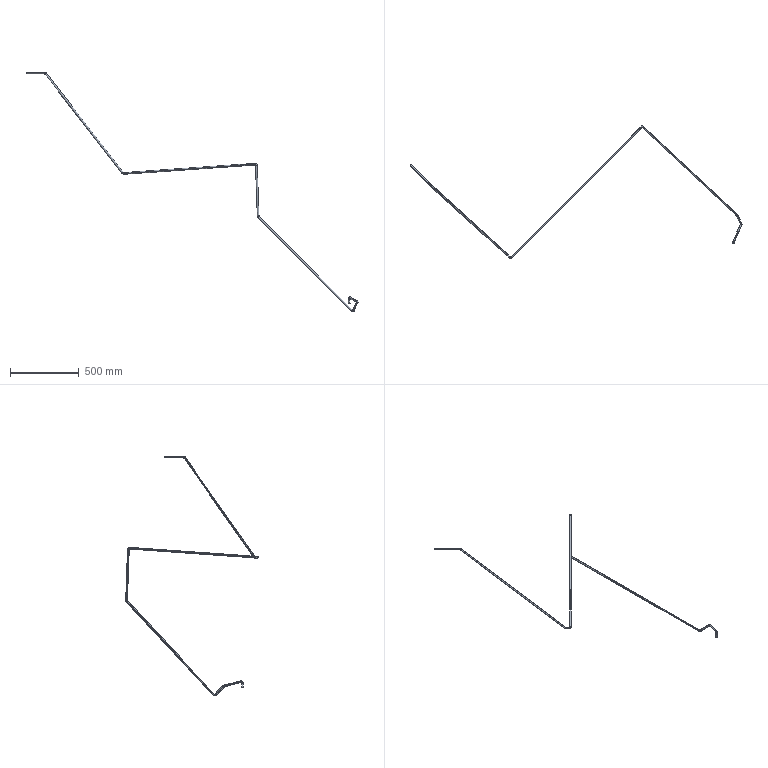Part | STEP file | Tube-500X083^Tube_4-P01_ASSEMBLY_KOMBAJN_OWOCOWYV11_Tube .500in OD X .083in Wall | 1 solid | 74 faces | box 2410 x 962.272 x 1741 mm | volume 310969 mm3 | torus 36 | cylinder 36 | plane 2 | commonest cylinder face diameters 8.484 x18 12.7 x18